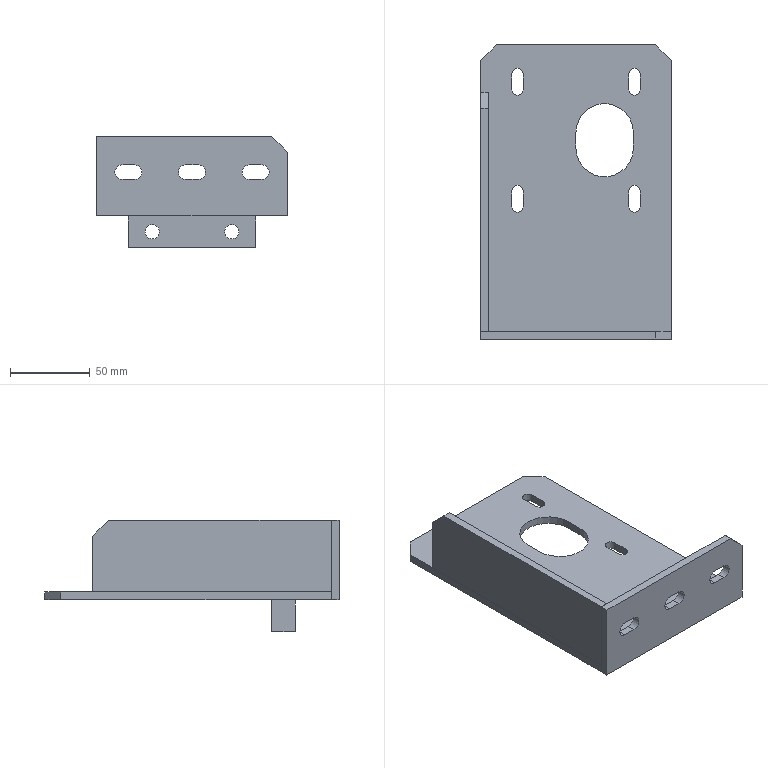Part | SolidWorks | features ICE 6, Chamfer 3, Extrusion 1 | 3 solids | 63 faces | box 120 x 185 x 70 mm | volume 181748 mm3 | plane 43 | cylinder 20 | commonest cylinder face diameters 9 x10 7 x8 36 x2